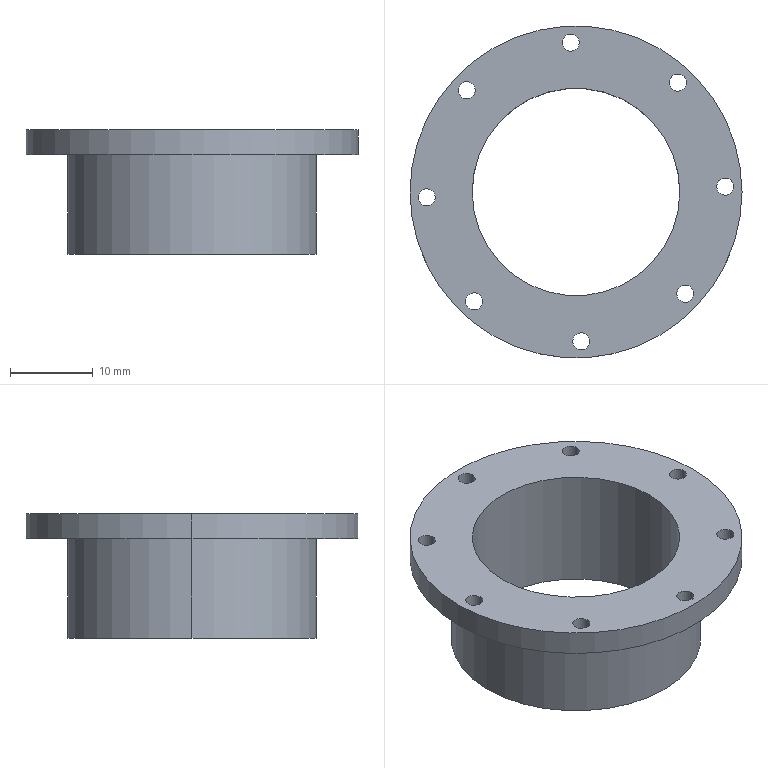Part | SolidWorks | features ICE 2, Cut 1, Extrusion 1 | 1 solid | 25 faces | box 40 x 40 x 15 mm | volume 4809 mm3 | cylinder 22 | plane 3 | commonest cylinder face diameters 2.06 x16 25 x2 30 x2 40 x2
STEP:
#1=CARTESIAN_POINT('',(16.959,0.6417,12.));
#2=VERTEX_POINT('',#1);
#3=CARTESIAN_POINT('',(19.019,0.6417,12.));
#4=VERTEX_POINT('',#3);
#5=CARTESIAN_POINT('',(17.989,0.6417,12.));
#6=DIRECTION('',(0.,0.,1.));
#7=DIRECTION('',(1.,0.,0.));
#8=AXIS2_PLACEMENT_3D('',#5,#6,#7);
#9=CIRCLE('',#8,1.03);
#10=EDGE_CURVE('',#2,#4,#9,.T.);
#11=ORIENTED_EDGE('',*,*,#10,.F.);
#12=CARTESIAN_POINT('',(16.959,0.6417,15.));
#13=VERTEX_POINT('',#12);
#14=CARTESIAN_POINT('',(16.959,0.6417,5.));
#15=DIRECTION('',(0.,0.,1.));
#16=VECTOR('',#15,1000.);
#17=LINE('',#14,#16);
#18=EDGE_CURVE('',#2,#13,#17,.T.);
#19=ORIENTED_EDGE('',*,*,#18,.T.);
#20=CARTESIAN_POINT('',(19.019,0.6417,15.));
#21=VERTEX_POINT('',#20);
#22=CARTESIAN_POINT('',(17.989,0.6417,15.));
#23=DIRECTION('',(0.,0.,1.));
#24=DIRECTION('',(1.,0.,0.));
#25=AXIS2_PLACEMENT_3D('',#22,#23,#24);
#26=CIRCLE('',#25,1.03);
#27=EDGE_CURVE('',#13,#21,#26,.T.);
#28=ORIENTED_EDGE('',*,*,#27,.T.);
#29=CARTESIAN_POINT('',(19.019,0.6417,5.));
#30=DIRECTION('',(0.,0.,1.));
#31=VECTOR('',#30,1000.);
#32=LINE('',#29,#31);
#33=EDGE_CURVE('',#4,#21,#32,.T.);
#34=ORIENTED_EDGE('',*,*,#33,.F.);
#35=EDGE_LOOP('',(#11,#19,#28,#34));
#36=FACE_OUTER_BOUND('',#35,.T.);
#37=CARTESIAN_POINT('',(17.989,0.6417,5.));
#38=DIRECTION('',(0.,0.,1.));
#39=DIRECTION('',(1.,0.,0.));
#40=AXIS2_PLACEMENT_3D('',#37,#38,#39);
#41=CYLINDRICAL_SURFACE('',#40,1.03);
#42=ADVANCED_FACE('',(#36),#41,.F.);
#43=CARTESIAN_POINT('',(12.144,-12.266,12.));
#44=VERTEX_POINT('',#43);
#45=CARTESIAN_POINT('',(14.204,-12.266,12.));
#46=VERTEX_POINT('',#45);
#47=CARTESIAN_POINT('',(13.174,-12.266,12.));
#48=DIRECTION('',(0.,0.,1.));
#49=DIRECTION('',(1.,0.,0.));
#50=AXIS2_PLACEMENT_3D('',#47,#48,#49);
#51=CIRCLE('',#50,1.03);
#52=EDGE_CURVE('',#44,#46,#51,.T.);
#53=ORIENTED_EDGE('',*,*,#52,.F.);
#54=CARTESIAN_POINT('',(12.144,-12.266,15.));
#55=VERTEX_POINT('',#54);
#56=CARTESIAN_POINT('',(12.144,-12.266,5.));
#57=DIRECTION('',(0.,0.,1.));
#58=VECTOR('',#57,1000.);
#59=LINE('',#56,#58);
#60=EDGE_CURVE('',#44,#55,#59,.T.);
#61=ORIENTED_EDGE('',*,*,#60,.T.);
#62=CARTESIAN_POINT('',(14.204,-12.266,15.));
#63=VERTEX_POINT('',#62);
#64=CARTESIAN_POINT('',(13.174,-12.266,15.));
#65=DIRECTION('',(0.,0.,1.));
#66=DIRECTION('',(1.,0.,0.));
#67=AXIS2_PLACEMENT_3D('',#64,#65,#66);
#68=CIRCLE('',#67,1.03);
#69=EDGE_CURVE('',#55,#63,#68,.T.);
#70=ORIENTED_EDGE('',*,*,#69,.T.);
#71=CARTESIAN_POINT('',(14.204,-12.266,5.));
#72=DIRECTION('',(0.,0.,1.));
#73=VECTOR('',#72,1000.);
#74=LINE('',#71,#73);
#75=EDGE_CURVE('',#46,#63,#74,.T.);
#76=ORIENTED_EDGE('',*,*,#75,.F.);
#77=EDGE_LOOP('',(#53,#61,#70,#76));
#78=FACE_OUTER_BOUND('',#77,.T.);
#79=CARTESIAN_POINT('',(13.174,-12.266,5.));
#80=DIRECTION('',(0.,0.,1.));
#81=DIRECTION('',(1.,0.,0.));
#82=AXIS2_PLACEMENT_3D('',#79,#80,#81);
#83=CYLINDRICAL_SURFACE('',#82,1.03);
#84=ADVANCED_FACE('',(#78),#83,.F.);
#85=CARTESIAN_POINT('',(-0.3883,-17.989,12.));
#86=VERTEX_POINT('',#85);
#87=CARTESIAN_POINT('',(1.672,-17.989,12.));
#88=VERTEX_POINT('',#87);
#89=CARTESIAN_POINT('',(0.6417,-17.989,12.));
#90=DIRECTION('',(0.,0.,1.));
#91=DIRECTION('',(1.,0.,0.));
#92=AXIS2_PLACEMENT_3D('',#89,#90,#91);
#93=CIRCLE('',#92,1.03);
#94=EDGE_CURVE('',#86,#88,#93,.T.);
#95=ORIENTED_EDGE('',*,*,#94,.F.);
#96=CARTESIAN_POINT('',(-0.3883,-17.989,15.));
#97=VERTEX_POINT('',#96);
#98=CARTESIAN_POINT('',(-0.3883,-17.989,5.));
#99=DIRECTION('',(0.,0.,1.));
#100=VECTOR('',#99,1000.);
#101=LINE('',#98,#100);
#102=EDGE_CURVE('',#86,#97,#101,.T.);
#103=ORIENTED_EDGE('',*,*,#102,.T.);
#104=CARTESIAN_POINT('',(1.672,-17.989,15.));
#105=VERTEX_POINT('',#104);
#106=CARTESIAN_POINT('',(0.6417,-17.989,15.));
#107=DIRECTION('',(0.,0.,1.));
#108=DIRECTION('',(1.,0.,0.));
#109=AXIS2_PLACEMENT_3D('',#106,#107,#108);
#110=CIRCLE('',#109,1.03);
#111=EDGE_CURVE('',#97,#105,#110,.T.);
#112=ORIENTED_EDGE('',*,*,#111,.T.);
#113=CARTESIAN_POINT('',(1.672,-17.989,5.));
#114=DIRECTION('',(0.,0.,1.));
#115=VECTOR('',#114,1000.);
#116=LINE('',#113,#115);
#117=EDGE_CURVE('',#88,#105,#116,.T.);
#118=ORIENTED_EDGE('',*,*,#117,.F.);
#119=EDGE_LOOP('',(#95,#103,#112,#118));
#120=FACE_OUTER_BOUND('',#119,.T.);
#121=CARTESIAN_POINT('',(0.6417,-17.989,5.));
#122=DIRECTION('',(0.,0.,1.));
#123=DIRECTION('',(1.,0.,0.));
#124=AXIS2_PLACEMENT_3D('',#121,#122,#123);
#125=CYLINDRICAL_SURFACE('',#124,1.03);
#126=ADVANCED_FACE('',(#120),#125,.F.);
#127=CARTESIAN_POINT('',(-13.296,-13.174,12.));
#128=VERTEX_POINT('',#127);
#129=CARTESIAN_POINT('',(-11.236,-13.174,12.));
#130=VERTEX_POINT('',#129);
#131=CARTESIAN_POINT('',(-12.266,-13.174,12.));
#132=DIRECTION('',(0.,0.,1.));
#133=DIRECTION('',(1.,0.,0.));
#134=AXIS2_PLACEMENT_3D('',#131,#132,#133);
#135=CIRCLE('',#134,1.03);
#136=EDGE_CURVE('',#128,#130,#135,.T.);
#137=ORIENTED_EDGE('',*,*,#136,.F.);
#138=CARTESIAN_POINT('',(-13.296,-13.174,15.));
#139=VERTEX_POINT('',#138);
#140=CARTESIAN_POINT('',(-13.296,-13.174,5.));
#141=DIRECTION('',(0.,0.,1.));
#142=VECTOR('',#141,1000.);
#143=LINE('',#140,#142);
#144=EDGE_CURVE('',#128,#139,#143,.T.);
#145=ORIENTED_EDGE('',*,*,#144,.T.);
#146=CARTESIAN_POINT('',(-11.236,-13.174,15.));
#147=VERTEX_POINT('',#146);
#148=CARTESIAN_POINT('',(-12.266,-13.174,15.));
#149=DIRECTION('',(0.,0.,1.));
#150=DIRECTION('',(1.,0.,0.));
#151=AXIS2_PLACEMENT_3D('',#148,#149,#150);
#152=CIRCLE('',#151,1.03);
#153=EDGE_CURVE('',#139,#147,#152,.T.);
#154=ORIENTED_EDGE('',*,*,#153,.T.);
#155=CARTESIAN_POINT('',(-11.236,-13.174,5.));
#156=DIRECTION('',(0.,0.,1.));
#157=VECTOR('',#156,1000.);
#158=LINE('',#155,#157);
#159=EDGE_CURVE('',#130,#147,#158,.T.);
#160=ORIENTED_EDGE('',*,*,#159,.F.);
#161=EDGE_LOOP('',(#137,#145,#154,#160));
#162=FACE_OUTER_BOUND('',#161,.T.);
#163=CARTESIAN_POINT('',(-12.266,-13.174,5.));
#164=DIRECTION('',(0.,0.,1.));
#165=DIRECTION('',(1.,0.,0.));
#166=AXIS2_PLACEMENT_3D('',#163,#164,#165);
#167=CYLINDRICAL_SURFACE('',#166,1.03);
#168=ADVANCED_FACE('',(#162),#167,.F.);
#169=CARTESIAN_POINT('',(-19.019,-0.6417,12.));
#170=VERTEX_POINT('',#169);
#171=CARTESIAN_POINT('',(-16.959,-0.6417,12.));
#172=VERTEX_POINT('',#171);
#173=CARTESIAN_POINT('',(-17.989,-0.6417,12.));
#174=DIRECTION('',(0.,0.,1.));
#175=DIRECTION('',(1.,0.,0.));
#176=AXIS2_PLACEMENT_3D('',#173,#174,#175);
#177=CIRCLE('',#176,1.03);
#178=EDGE_CURVE('',#170,#172,#177,.T.);
#179=ORIENTED_EDGE('',*,*,#178,.F.);
#180=CARTESIAN_POINT('',(-19.019,-0.6417,15.));
#181=VERTEX_POINT('',#180);
#182=CARTESIAN_POINT('',(-19.019,-0.6417,5.));
#183=DIRECTION('',(0.,0.,1.));
#184=VECTOR('',#183,1000.);
#185=LINE('',#182,#184);
#186=EDGE_CURVE('',#170,#181,#185,.T.);
#187=ORIENTED_EDGE('',*,*,#186,.T.);
#188=CARTESIAN_POINT('',(-16.959,-0.6417,15.));
#189=VERTEX_POINT('',#188);
#190=CARTESIAN_POINT('',(-17.989,-0.6417,15.));
#191=DIRECTION('',(0.,0.,1.));
#192=DIRECTION('',(1.,0.,0.));
#193=AXIS2_PLACEMENT_3D('',#190,#191,#192);
#194=CIRCLE('',#193,1.03);
#195=EDGE_CURVE('',#181,#189,#194,.T.);
#196=ORIENTED_EDGE('',*,*,#195,.T.);
#197=CARTESIAN_POINT('',(-16.959,-0.6417,5.));
#198=DIRECTION('',(0.,0.,1.));
#199=VECTOR('',#198,1000.);
#200=LINE('',#197,#199);
#201=EDGE_CURVE('',#172,#189,#200,.T.);
#202=ORIENTED_EDGE('',*,*,#201,.F.);
#203=EDGE_LOOP('',(#179,#187,#196,#202));
#204=FACE_OUTER_BOUND('',#203,.T.);
#205=CARTESIAN_POINT('',(-17.989,-0.6417,5.));
#206=DIRECTION('',(0.,0.,1.));
#207=DIRECTION('',(1.,0.,0.));
#208=AXIS2_PLACEMENT_3D('',#205,#206,#207);
#209=CYLINDRICAL_SURFACE('',#208,1.03);
#210=ADVANCED_FACE('',(#204),#209,.F.);
#211=CARTESIAN_POINT('',(-14.204,12.266,12.));
#212=VERTEX_POINT('',#211);
#213=CARTESIAN_POINT('',(-12.144,12.266,12.));
#214=VERTEX_POINT('',#213);
#215=CARTESIAN_POINT('',(-13.174,12.266,12.));
#216=DIRECTION('',(0.,0.,1.));
#217=DIRECTION('',(1.,0.,0.));
#218=AXIS2_PLACEMENT_3D('',#215,#216,#217);
#219=CIRCLE('',#218,1.03);
#220=EDGE_CURVE('',#212,#214,#219,.T.);
#221=ORIENTED_EDGE('',*,*,#220,.F.);
#222=CARTESIAN_POINT('',(-14.204,12.266,15.));
#223=VERTEX_POINT('',#222);
#224=CARTESIAN_POINT('',(-14.204,12.266,5.));
#225=DIRECTION('',(0.,0.,1.));
#226=VECTOR('',#225,1000.);
#227=LINE('',#224,#226);
#228=EDGE_CURVE('',#212,#223,#227,.T.);
#229=ORIENTED_EDGE('',*,*,#228,.T.);
#230=CARTESIAN_POINT('',(-12.144,12.266,15.));
#231=VERTEX_POINT('',#230);
#232=CARTESIAN_POINT('',(-13.174,12.266,15.));
#233=DIRECTION('',(0.,0.,1.));
#234=DIRECTION('',(1.,0.,0.));
#235=AXIS2_PLACEMENT_3D('',#232,#233,#234);
#236=CIRCLE('',#235,1.03);
#237=EDGE_CURVE('',#223,#231,#236,.T.);
#238=ORIENTED_EDGE('',*,*,#237,.T.);
#239=CARTESIAN_POINT('',(-12.144,12.266,5.));
#240=DIRECTION('',(0.,0.,1.));
#241=VECTOR('',#240,1000.);
#242=LINE('',#239,#241);
#243=EDGE_CURVE('',#214,#231,#242,.T.);
#244=ORIENTED_EDGE('',*,*,#243,.F.);
#245=EDGE_LOOP('',(#221,#229,#238,#244));
#246=FACE_OUTER_BOUND('',#245,.T.);
#247=CARTESIAN_POINT('',(-13.174,12.266,5.));
#248=DIRECTION('',(0.,0.,1.));
#249=DIRECTION('',(1.,0.,0.));
#250=AXIS2_PLACEMENT_3D('',#247,#248,#249);
#251=CYLINDRICAL_SURFACE('',#250,1.03);
#252=ADVANCED_FACE('',(#246),#251,.F.);
#253=CARTESIAN_POINT('',(-1.672,17.989,12.));
#254=VERTEX_POINT('',#253);
#255=CARTESIAN_POINT('',(0.3883,17.989,12.));
#256=VERTEX_POINT('',#255);
#257=CARTESIAN_POINT('',(-0.6417,17.989,12.));
#258=DIRECTION('',(0.,0.,1.));
#259=DIRECTION('',(1.,0.,0.));
#260=AXIS2_PLACEMENT_3D('',#257,#258,#259);
#261=CIRCLE('',#260,1.03);
#262=EDGE_CURVE('',#254,#256,#261,.T.);
#263=ORIENTED_EDGE('',*,*,#262,.F.);
#264=CARTESIAN_POINT('',(-1.672,17.989,15.));
#265=VERTEX_POINT('',#264);
#266=CARTESIAN_POINT('',(-1.672,17.989,5.));
#267=DIRECTION('',(0.,0.,1.));
#268=VECTOR('',#267,1000.);
#269=LINE('',#266,#268);
#270=EDGE_CURVE('',#254,#265,#269,.T.);
#271=ORIENTED_EDGE('',*,*,#270,.T.);
#272=CARTESIAN_POINT('',(0.3883,17.989,15.));
#273=VERTEX_POINT('',#272);
#274=CARTESIAN_POINT('',(-0.6417,17.989,15.));
#275=DIRECTION('',(0.,0.,1.));
#276=DIRECTION('',(1.,0.,0.));
#277=AXIS2_PLACEMENT_3D('',#274,#275,#276);
#278=CIRCLE('',#277,1.03);
#279=EDGE_CURVE('',#265,#273,#278,.T.);
#280=ORIENTED_EDGE('',*,*,#279,.T.);
#281=CARTESIAN_POINT('',(0.3883,17.989,5.));
#282=DIRECTION('',(0.,0.,1.));
#283=VECTOR('',#282,1000.);
#284=LINE('',#281,#283);
#285=EDGE_CURVE('',#256,#273,#284,.T.);
#286=ORIENTED_EDGE('',*,*,#285,.F.);
#287=EDGE_LOOP('',(#263,#271,#280,#286));
#288=FACE_OUTER_BOUND('',#287,.T.);
#289=CARTESIAN_POINT('',(-0.6417,17.989,5.));
#290=DIRECTION('',(0.,0.,1.));
#291=DIRECTION('',(1.,0.,0.));
#292=AXIS2_PLACEMENT_3D('',#289,#290,#291);
#293=CYLINDRICAL_SURFACE('',#292,1.03);
#294=ADVANCED_FACE('',(#288),#293,.F.);
#295=CARTESIAN_POINT('',(11.236,13.174,12.));
#296=VERTEX_POINT('',#295);
#297=CARTESIAN_POINT('',(13.296,13.174,12.));
#298=VERTEX_POINT('',#297);
#299=CARTESIAN_POINT('',(12.266,13.174,12.));
#300=DIRECTION('',(0.,0.,1.));
#301=DIRECTION('',(1.,0.,0.));
#302=AXIS2_PLACEMENT_3D('',#299,#300,#301);
#303=CIRCLE('',#302,1.03);
#304=EDGE_CURVE('',#296,#298,#303,.T.);
#305=ORIENTED_EDGE('',*,*,#304,.F.);
#306=CARTESIAN_POINT('',(11.236,13.174,15.));
#307=VERTEX_POINT('',#306);
#308=CARTESIAN_POINT('',(11.236,13.174,5.));
#309=DIRECTION('',(0.,0.,1.));
#310=VECTOR('',#309,1000.);
#311=LINE('',#308,#310);
#312=EDGE_CURVE('',#296,#307,#311,.T.);
#313=ORIENTED_EDGE('',*,*,#312,.T.);
#314=CARTESIAN_POINT('',(13.296,13.174,15.));
#315=VERTEX_POINT('',#314);
#316=CARTESIAN_POINT('',(12.266,13.174,15.));
#317=DIRECTION('',(0.,0.,1.));
#318=DIRECTION('',(1.,0.,0.));
#319=AXIS2_PLACEMENT_3D('',#316,#317,#318);
#320=CIRCLE('',#319,1.03);
#321=EDGE_CURVE('',#307,#315,#320,.T.);
#322=ORIENTED_EDGE('',*,*,#321,.T.);
#323=CARTESIAN_POINT('',(13.296,13.174,5.));
#324=DIRECTION('',(0.,0.,1.));
#325=VECTOR('',#324,1000.);
#326=LINE('',#323,#325);
#327=EDGE_CURVE('',#298,#315,#326,.T.);
#328=ORIENTED_EDGE('',*,*,#327,.F.);
#329=EDGE_LOOP('',(#305,#313,#322,#328));
#330=FACE_OUTER_BOUND('',#329,.T.);
#331=CARTESIAN_POINT('',(12.266,13.174,5.));
#332=DIRECTION('',(0.,0.,1.));
#333=DIRECTION('',(1.,0.,0.));
#334=AXIS2_PLACEMENT_3D('',#331,#332,#333);
#335=CYLINDRICAL_SURFACE('',#334,1.03);
#336=ADVANCED_FACE('',(#330),#335,.F.);
#337=CARTESIAN_POINT('',(20.,0.,15.));
#338=VERTEX_POINT('',#337);
#339=CARTESIAN_POINT('',(-20.,0.,15.));
#340=VERTEX_POINT('',#339);
#341=CARTESIAN_POINT('',(0.,0.,15.));
#342=DIRECTION('',(0.,0.,1.));
#343=DIRECTION('',(1.,0.,0.));
#344=AXIS2_PLACEMENT_3D('',#341,#342,#343);
#345=CIRCLE('',#344,20.);
#346=EDGE_CURVE('',#338,#340,#345,.T.);
#347=ORIENTED_EDGE('',*,*,#346,.F.);
#348=CARTESIAN_POINT('',(20.,0.,12.));
#349=VERTEX_POINT('',#348);
#350=CARTESIAN_POINT('',(20.,0.,71.569));
#351=DIRECTION('',(0.,0.,-1.));
#352=VECTOR('',#351,1000.);
#353=LINE('',#350,#352);
#354=EDGE_CURVE('',#338,#349,#353,.T.);
#355=ORIENTED_EDGE('',*,*,#354,.T.);
#356=CARTESIAN_POINT('',(-20.,0.,12.));
#357=VERTEX_POINT('',#356);
#358=CARTESIAN_POINT('',(0.,0.,12.));
#359=DIRECTION('',(0.,0.,1.));
#360=DIRECTION('',(1.,0.,0.));
#361=AXIS2_PLACEMENT_3D('',#358,#359,#360);
#362=CIRCLE('',#361,20.);
#363=EDGE_CURVE('',#349,#357,#362,.T.);
#364=ORIENTED_EDGE('',*,*,#363,.T.);
#365=CARTESIAN_POINT('',(-20.,0.,71.569));
#366=DIRECTION('',(0.,0.,-1.));
#367=VECTOR('',#366,1000.);
#368=LINE('',#365,#367);
#369=EDGE_CURVE('',#340,#357,#368,.T.);
#370=ORIENTED_EDGE('',*,*,#369,.F.);
#371=EDGE_LOOP('',(#347,#355,#364,#370));
#372=FACE_OUTER_BOUND('',#371,.T.);
#373=CARTESIAN_POINT('',(0.,0.,71.569));
#374=DIRECTION('',(0.,0.,-1.));
#375=DIRECTION('',(-1.,0.,0.));
#376=AXIS2_PLACEMENT_3D('',#373,#374,#375);
#377=CYLINDRICAL_SURFACE('',#376,20.);
#378=ADVANCED_FACE('',(#372),#377,.T.);
#379=CARTESIAN_POINT('',(-12.5,0.,15.));
#380=VERTEX_POINT('',#379);
#381=CARTESIAN_POINT('',(12.5,0.,15.));
#382=VERTEX_POINT('',#381);
#383=CARTESIAN_POINT('',(0.,0.,15.));
#384=DIRECTION('',(0.,0.,1.));
#385=DIRECTION('',(1.,0.,0.));
#386=AXIS2_PLACEMENT_3D('',#383,#384,#385);
#387=CIRCLE('',#386,12.5);
#388=EDGE_CURVE('',#380,#382,#387,.T.);
#389=ORIENTED_EDGE('',*,*,#388,.T.);
#390=CARTESIAN_POINT('',(12.5,0.,0.));
#391=VERTEX_POINT('',#390);
#392=CARTESIAN_POINT('',(12.5,0.,5.));
#393=DIRECTION('',(0.,0.,-1.));
#394=VECTOR('',#393,1000.);
#395=LINE('',#392,#394);
#396=EDGE_CURVE('',#382,#391,#395,.T.);
#397=ORIENTED_EDGE('',*,*,#396,.T.);
#398=CARTESIAN_POINT('',(-12.5,0.,0.));
#399=VERTEX_POINT('',#398);
#400=CARTESIAN_POINT('',(0.,0.,0.));
#401=DIRECTION('',(0.,0.,1.));
#402=DIRECTION('',(1.,0.,0.));
#403=AXIS2_PLACEMENT_3D('',#400,#401,#402);
#404=CIRCLE('',#403,12.5);
#405=EDGE_CURVE('',#399,#391,#404,.T.);
#406=ORIENTED_EDGE('',*,*,#405,.F.);
#407=CARTESIAN_POINT('',(-12.5,0.,5.));
#408=DIRECTION('',(0.,0.,-1.));
#409=VECTOR('',#408,1000.);
#410=LINE('',#407,#409);
#411=EDGE_CURVE('',#380,#399,#410,.T.);
#412=ORIENTED_EDGE('',*,*,#411,.F.);
#413=EDGE_LOOP('',(#389,#397,#406,#412));
#414=FACE_OUTER_BOUND('',#413,.T.);
#415=CARTESIAN_POINT('',(0.,0.,5.));
#416=DIRECTION('',(0.,0.,-1.));
#417=DIRECTION('',(-1.,0.,0.));
#418=AXIS2_PLACEMENT_3D('',#415,#416,#417);
#419=CYLINDRICAL_SURFACE('',#418,12.5);
#420=ADVANCED_FACE('',(#414),#419,.F.);
#421=CARTESIAN_POINT('',(15.,0.,12.));
#422=VERTEX_POINT('',#421);
#423=CARTESIAN_POINT('',(-15.,0.,12.));
#424=VERTEX_POINT('',#423);
#425=CARTESIAN_POINT('',(0.,0.,12.));
#426=DIRECTION('',(0.,0.,1.));
#427=DIRECTION('',(1.,0.,0.));
#428=AXIS2_PLACEMENT_3D('',#425,#426,#427);
#429=CIRCLE('',#428,15.);
#430=EDGE_CURVE('',#422,#424,#429,.T.);
#431=ORIENTED_EDGE('',*,*,#430,.F.);
#432=CARTESIAN_POINT('',(15.,0.,0.));
#433=VERTEX_POINT('',#432);
#434=CARTESIAN_POINT('',(15.,0.,5.));
#435=DIRECTION('',(0.,0.,-1.));
#436=VECTOR('',#435,1000.);
#437=LINE('',#434,#436);
#438=EDGE_CURVE('',#422,#433,#437,.T.);
#439=ORIENTED_EDGE('',*,*,#438,.T.);
#440=CARTESIAN_POINT('',(-15.,0.,0.));
#441=VERTEX_POINT('',#440);
#442=CARTESIAN_POINT('',(0.,0.,0.));
#443=DIRECTION('',(0.,0.,1.));
#444=DIRECTION('',(1.,0.,0.));
#445=AXIS2_PLACEMENT_3D('',#442,#443,#444);
#446=CIRCLE('',#445,15.);
#447=EDGE_CURVE('',#433,#441,#446,.T.);
#448=ORIENTED_EDGE('',*,*,#447,.T.);
#449=CARTESIAN_POINT('',(-15.,0.,5.));
#450=DIRECTION('',(0.,0.,-1.));
#451=VECTOR('',#450,1000.);
#452=LINE('',#449,#451);
#453=EDGE_CURVE('',#424,#441,#452,.T.);
#454=ORIENTED_EDGE('',*,*,#453,.F.);
#455=EDGE_LOOP('',(#431,#439,#448,#454));
#456=FACE_OUTER_BOUND('',#455,.T.);
#457=CARTESIAN_POINT('',(0.,0.,5.));
#458=DIRECTION('',(0.,0.,-1.));
#459=DIRECTION('',(-1.,0.,0.));
#460=AXIS2_PLACEMENT_3D('',#457,#458,#459);
#461=CYLINDRICAL_SURFACE('',#460,15.);
#462=ADVANCED_FACE('',(#456),#461,.T.);
#463=ORIENTED_EDGE('',*,*,#438,.F.);
#464=CARTESIAN_POINT('',(0.,0.,12.));
#465=DIRECTION('',(0.,0.,1.));
#466=DIRECTION('',(1.,0.,0.));
#467=AXIS2_PLACEMENT_3D('',#464,#465,#466);
#468=CIRCLE('',#467,15.);
#469=EDGE_CURVE('',#424,#422,#468,.T.);
#470=ORIENTED_EDGE('',*,*,#469,.F.);
#471=ORIENTED_EDGE('',*,*,#453,.T.);
#472=CARTESIAN_POINT('',(0.,0.,0.));
#473=DIRECTION('',(0.,0.,1.));
#474=DIRECTION('',(1.,0.,0.));
#475=AXIS2_PLACEMENT_3D('',#472,#473,#474);
#476=CIRCLE('',#475,15.);
#477=EDGE_CURVE('',#441,#433,#476,.T.);
#478=ORIENTED_EDGE('',*,*,#477,.T.);
#479=EDGE_LOOP('',(#463,#470,#471,#478));
#480=FACE_OUTER_BOUND('',#479,.T.);
#481=CARTESIAN_POINT('',(0.,0.,5.));
#482=DIRECTION('',(0.,0.,-1.));
#483=DIRECTION('',(-1.,0.,0.));
#484=AXIS2_PLACEMENT_3D('',#481,#482,#483);
#485=CYLINDRICAL_SURFACE('',#484,15.);
#486=ADVANCED_FACE('',(#480),#485,.T.);
#487=ORIENTED_EDGE('',*,*,#477,.F.);
#488=ORIENTED_EDGE('',*,*,#447,.F.);
#489=EDGE_LOOP('',(#487,#488));
#490=FACE_OUTER_BOUND('',#489,.T.);
#491=ORIENTED_EDGE('',*,*,#405,.T.);
#492=CARTESIAN_POINT('',(0.,0.,0.));
#493=DIRECTION('',(0.,0.,1.));
#494=DIRECTION('',(1.,0.,0.));
#495=AXIS2_PLACEMENT_3D('',#492,#493,#494);
#496=CIRCLE('',#495,12.5);
#497=EDGE_CURVE('',#391,#399,#496,.T.);
#498=ORIENTED_EDGE('',*,*,#497,.T.);
#499=EDGE_LOOP('',(#491,#498));
#500=FACE_BOUND('',#499,.T.);
#501=CARTESIAN_POINT('',(0.,0.,0.));
#502=DIRECTION('',(0.,0.,1.));
#503=DIRECTION('',(1.,0.,0.));
#504=AXIS2_PLACEMENT_3D('',#501,#502,#503);
#505=PLANE('',#504);
#506=ADVANCED_FACE('',(#490,#500),#505,.F.);
#507=ORIENTED_EDGE('',*,*,#396,.F.);
#508=CARTESIAN_POINT('',(0.,0.,15.));
#509=DIRECTION('',(0.,0.,1.));
#510=DIRECTION('',(1.,0.,0.));
#511=AXIS2_PLACEMENT_3D('',#508,#509,#510);
#512=CIRCLE('',#511,12.5);
#513=EDGE_CURVE('',#382,#380,#512,.T.);
#514=ORIENTED_EDGE('',*,*,#513,.T.);
#515=ORIENTED_EDGE('',*,*,#411,.T.);
#516=ORIENTED_EDGE('',*,*,#497,.F.);
#517=EDGE_LOOP('',(#507,#514,#515,#516));
#518=FACE_OUTER_BOUND('',#517,.T.);
#519=CARTESIAN_POINT('',(0.,0.,5.));
#520=DIRECTION('',(0.,0.,-1.));
#521=DIRECTION('',(-1.,0.,0.));
#522=AXIS2_PLACEMENT_3D('',#519,#520,#521);
#523=CYLINDRICAL_SURFACE('',#522,12.5);
#524=ADVANCED_FACE('',(#518),#523,.F.);
#525=CARTESIAN_POINT('',(17.989,0.6417,15.));
#526=DIRECTION('',(0.,0.,1.));
#527=DIRECTION('',(1.,0.,0.));
#528=AXIS2_PLACEMENT_3D('',#525,#526,#527);
#529=CIRCLE('',#528,1.03);
#530=EDGE_CURVE('',#21,#13,#529,.T.);
#531=ORIENTED_EDGE('',*,*,#530,.F.);
#532=ORIENTED_EDGE('',*,*,#27,.F.);
#533=EDGE_LOOP('',(#531,#532));
#534=FACE_BOUND('',#533,.T.);
#535=CARTESIAN_POINT('',(13.174,-12.266,15.));
#536=DIRECTION('',(0.,0.,1.));
#537=DIRECTION('',(1.,0.,0.));
#538=AXIS2_PLACEMENT_3D('',#535,#536,#537);
#539=CIRCLE('',#538,1.03);
#540=EDGE_CURVE('',#63,#55,#539,.T.);
#541=ORIENTED_EDGE('',*,*,#540,.F.);
#542=ORIENTED_EDGE('',*,*,#69,.F.);
#543=EDGE_LOOP('',(#541,#542));
#544=FACE_BOUND('',#543,.T.);
#545=CARTESIAN_POINT('',(0.6417,-17.989,15.));
#546=DIRECTION('',(0.,0.,1.));
#547=DIRECTION('',(1.,0.,0.));
#548=AXIS2_PLACEMENT_3D('',#545,#546,#547);
#549=CIRCLE('',#548,1.03);
#550=EDGE_CURVE('',#105,#97,#549,.T.);
#551=ORIENTED_EDGE('',*,*,#550,.F.);
#552=ORIENTED_EDGE('',*,*,#111,.F.);
#553=EDGE_LOOP('',(#551,#552));
#554=FACE_BOUND('',#553,.T.);
#555=CARTESIAN_POINT('',(-12.266,-13.174,15.));
#556=DIRECTION('',(0.,0.,1.));
#557=DIRECTION('',(1.,0.,0.));
#558=AXIS2_PLACEMENT_3D('',#555,#556,#557);
#559=CIRCLE('',#558,1.03);
#560=EDGE_CURVE('',#147,#139,#559,.T.);
#561=ORIENTED_EDGE('',*,*,#560,.F.);
#562=ORIENTED_EDGE('',*,*,#153,.F.);
#563=EDGE_LOOP('',(#561,#562));
#564=FACE_BOUND('',#563,.T.);
#565=CARTESIAN_POINT('',(-17.989,-0.6417,15.));
#566=DIRECTION('',(0.,0.,1.));
#567=DIRECTION('',(1.,0.,0.));
#568=AXIS2_PLACEMENT_3D('',#565,#566,#567);
#569=CIRCLE('',#568,1.03);
#570=EDGE_CURVE('',#189,#181,#569,.T.);
#571=ORIENTED_EDGE('',*,*,#570,.F.);
#572=ORIENTED_EDGE('',*,*,#195,.F.);
#573=EDGE_LOOP('',(#571,#572));
#574=FACE_BOUND('',#573,.T.);
#575=CARTESIAN_POINT('',(-13.174,12.266,15.));
#576=DIRECTION('',(0.,0.,1.));
#577=DIRECTION('',(1.,0.,0.));
#578=AXIS2_PLACEMENT_3D('',#575,#576,#577);
#579=CIRCLE('',#578,1.03);
#580=EDGE_CURVE('',#231,#223,#579,.T.);
#581=ORIENTED_EDGE('',*,*,#580,.F.);
#582=ORIENTED_EDGE('',*,*,#237,.F.);
#583=EDGE_LOOP('',(#581,#582));
#584=FACE_BOUND('',#583,.T.);
#585=CARTESIAN_POINT('',(-0.6417,17.989,15.));
#586=DIRECTION('',(0.,0.,1.));
#587=DIRECTION('',(1.,0.,0.));
#588=AXIS2_PLACEMENT_3D('',#585,#586,#587);
#589=CIRCLE('',#588,1.03);
#590=EDGE_CURVE('',#273,#265,#589,.T.);
#591=ORIENTED_EDGE('',*,*,#590,.F.);
#592=ORIENTED_EDGE('',*,*,#279,.F.);
#593=EDGE_LOOP('',(#591,#592));
#594=FACE_BOUND('',#593,.T.);
#595=CARTESIAN_POINT('',(12.266,13.174,15.));
#596=DIRECTION('',(0.,0.,1.));
#597=DIRECTION('',(1.,0.,0.));
#598=AXIS2_PLACEMENT_3D('',#595,#596,#597);
#599=CIRCLE('',#598,1.03);
#600=EDGE_CURVE('',#315,#307,#599,.T.);
#601=ORIENTED_EDGE('',*,*,#600,.F.);
#602=ORIENTED_EDGE('',*,*,#321,.F.);
#603=EDGE_LOOP('',(#601,#602));
#604=FACE_BOUND('',#603,.T.);
#605=ORIENTED_EDGE('',*,*,#388,.F.);
#606=ORIENTED_EDGE('',*,*,#513,.F.);
#607=EDGE_LOOP('',(#605,#606));
#608=FACE_BOUND('',#607,.T.);
#609=CARTESIAN_POINT('',(0.,0.,15.));
#610=DIRECTION('',(0.,0.,1.));
#611=DIRECTION('',(1.,0.,0.));
#612=AXIS2_PLACEMENT_3D('',#609,#610,#611);
#613=CIRCLE('',#612,20.);
#614=EDGE_CURVE('',#340,#338,#613,.T.);
#615=ORIENTED_EDGE('',*,*,#614,.T.);
#616=ORIENTED_EDGE('',*,*,#346,.T.);
#617=EDGE_LOOP('',(#615,#616));
#618=FACE_OUTER_BOUND('',#617,.T.);
#619=CARTESIAN_POINT('',(0.,0.,15.));
#620=DIRECTION('',(0.,0.,1.));
#621=DIRECTION('',(1.,0.,0.));
#622=AXIS2_PLACEMENT_3D('',#619,#620,#621);
#623=PLANE('',#622);
#624=ADVANCED_FACE('',(#534,#544,#554,#564,#574,#584,#594,#604,#608,#618),#623,.T.);
#625=ORIENTED_EDGE('',*,*,#354,.F.);
#626=ORIENTED_EDGE('',*,*,#614,.F.);
#627=ORIENTED_EDGE('',*,*,#369,.T.);
#628=CARTESIAN_POINT('',(0.,0.,12.));
#629=DIRECTION('',(0.,0.,1.));
#630=DIRECTION('',(1.,0.,0.));
#631=AXIS2_PLACEMENT_3D('',#628,#629,#630);
#632=CIRCLE('',#631,20.);
#633=EDGE_CURVE('',#357,#349,#632,.T.);
#634=ORIENTED_EDGE('',*,*,#633,.T.);
#635=EDGE_LOOP('',(#625,#626,#627,#634));
#636=FACE_OUTER_BOUND('',#635,.T.);
#637=CARTESIAN_POINT('',(0.,0.,71.569));
#638=DIRECTION('',(0.,0.,-1.));
#639=DIRECTION('',(-1.,0.,0.));
#640=AXIS2_PLACEMENT_3D('',#637,#638,#639);
#641=CYLINDRICAL_SURFACE('',#640,20.);
#642=ADVANCED_FACE('',(#636),#641,.T.);
#643=CARTESIAN_POINT('',(17.989,0.6417,12.));
#644=DIRECTION('',(0.,0.,1.));
#645=DIRECTION('',(1.,0.,0.));
#646=AXIS2_PLACEMENT_3D('',#643,#644,#645);
#647=CIRCLE('',#646,1.03);
#648=EDGE_CURVE('',#4,#2,#647,.T.);
#649=ORIENTED_EDGE('',*,*,#648,.T.);
#650=ORIENTED_EDGE('',*,*,#10,.T.);
#651=EDGE_LOOP('',(#649,#650));
#652=FACE_BOUND('',#651,.T.);
#653=CARTESIAN_POINT('',(13.174,-12.266,12.));
#654=DIRECTION('',(0.,0.,1.));
#655=DIRECTION('',(1.,0.,0.));
#656=AXIS2_PLACEMENT_3D('',#653,#654,#655);
#657=CIRCLE('',#656,1.03);
#658=EDGE_CURVE('',#46,#44,#657,.T.);
#659=ORIENTED_EDGE('',*,*,#658,.T.);
#660=ORIENTED_EDGE('',*,*,#52,.T.);
#661=EDGE_LOOP('',(#659,#660));
#662=FACE_BOUND('',#661,.T.);
#663=CARTESIAN_POINT('',(0.6417,-17.989,12.));
#664=DIRECTION('',(0.,0.,1.));
#665=DIRECTION('',(1.,0.,0.));
#666=AXIS2_PLACEMENT_3D('',#663,#664,#665);
#667=CIRCLE('',#666,1.03);
#668=EDGE_CURVE('',#88,#86,#667,.T.);
#669=ORIENTED_EDGE('',*,*,#668,.T.);
#670=ORIENTED_EDGE('',*,*,#94,.T.);
#671=EDGE_LOOP('',(#669,#670));
#672=FACE_BOUND('',#671,.T.);
#673=CARTESIAN_POINT('',(-12.266,-13.174,12.));
#674=DIRECTION('',(0.,0.,1.));
#675=DIRECTION('',(1.,0.,0.));
#676=AXIS2_PLACEMENT_3D('',#673,#674,#675);
#677=CIRCLE('',#676,1.03);
#678=EDGE_CURVE('',#130,#128,#677,.T.);
#679=ORIENTED_EDGE('',*,*,#678,.T.);
#680=ORIENTED_EDGE('',*,*,#136,.T.);
#681=EDGE_LOOP('',(#679,#680));
#682=FACE_BOUND('',#681,.T.);
#683=CARTESIAN_POINT('',(-17.989,-0.6417,12.));
#684=DIRECTION('',(0.,0.,1.));
#685=DIRECTION('',(1.,0.,0.));
#686=AXIS2_PLACEMENT_3D('',#683,#684,#685);
#687=CIRCLE('',#686,1.03);
#688=EDGE_CURVE('',#172,#170,#687,.T.);
#689=ORIENTED_EDGE('',*,*,#688,.T.);
#690=ORIENTED_EDGE('',*,*,#178,.T.);
#691=EDGE_LOOP('',(#689,#690));
#692=FACE_BOUND('',#691,.T.);
#693=CARTESIAN_POINT('',(-13.174,12.266,12.));
#694=DIRECTION('',(0.,0.,1.));
#695=DIRECTION('',(1.,0.,0.));
#696=AXIS2_PLACEMENT_3D('',#693,#694,#695);
#697=CIRCLE('',#696,1.03);
#698=EDGE_CURVE('',#214,#212,#697,.T.);
#699=ORIENTED_EDGE('',*,*,#698,.T.);
#700=ORIENTED_EDGE('',*,*,#220,.T.);
#701=EDGE_LOOP('',(#699,#700));
#702=FACE_BOUND('',#701,.T.);
#703=CARTESIAN_POINT('',(-0.6417,17.989,12.));
#704=DIRECTION('',(0.,0.,1.));
#705=DIRECTION('',(1.,0.,0.));
#706=AXIS2_PLACEMENT_3D('',#703,#704,#705);
#707=CIRCLE('',#706,1.03);
#708=EDGE_CURVE('',#256,#254,#707,.T.);
#709=ORIENTED_EDGE('',*,*,#708,.T.);
#710=ORIENTED_EDGE('',*,*,#262,.T.);
#711=EDGE_LOOP('',(#709,#710));
#712=FACE_BOUND('',#711,.T.);
#713=CARTESIAN_POINT('',(12.266,13.174,12.));
#714=DIRECTION('',(0.,0.,1.));
#715=DIRECTION('',(1.,0.,0.));
#716=AXIS2_PLACEMENT_3D('',#713,#714,#715);
#717=CIRCLE('',#716,1.03);
#718=EDGE_CURVE('',#298,#296,#717,.T.);
#719=ORIENTED_EDGE('',*,*,#718,.T.);
#720=ORIENTED_EDGE('',*,*,#304,.T.);
#721=EDGE_LOOP('',(#719,#720));
#722=FACE_BOUND('',#721,.T.);
#723=ORIENTED_EDGE('',*,*,#469,.T.);
#724=ORIENTED_EDGE('',*,*,#430,.T.);
#725=EDGE_LOOP('',(#723,#724));
#726=FACE_BOUND('',#725,.T.);
#727=ORIENTED_EDGE('',*,*,#633,.F.);
#728=ORIENTED_EDGE('',*,*,#363,.F.);
#729=EDGE_LOOP('',(#727,#728));
#730=FACE_OUTER_BOUND('',#729,.T.);
#731=CARTESIAN_POINT('',(0.,0.,12.));
#732=DIRECTION('',(0.,0.,1.));
#733=DIRECTION('',(1.,0.,0.));
#734=AXIS2_PLACEMENT_3D('',#731,#732,#733);
#735=PLANE('',#734);
#736=ADVANCED_FACE('',(#652,#662,#672,#682,#692,#702,#712,#722,#726,#730),#735,.F.);
#737=ORIENTED_EDGE('',*,*,#312,.F.);
#738=ORIENTED_EDGE('',*,*,#718,.F.);
#739=ORIENTED_EDGE('',*,*,#327,.T.);
#740=ORIENTED_EDGE('',*,*,#600,.T.);
#741=EDGE_LOOP('',(#737,#738,#739,#740));
#742=FACE_OUTER_BOUND('',#741,.T.);
#743=CARTESIAN_POINT('',(12.266,13.174,5.));
#744=DIRECTION('',(0.,0.,1.));
#745=DIRECTION('',(1.,0.,0.));
#746=AXIS2_PLACEMENT_3D('',#743,#744,#745);
#747=CYLINDRICAL_SURFACE('',#746,1.03);
#748=ADVANCED_FACE('',(#742),#747,.F.);
#749=ORIENTED_EDGE('',*,*,#270,.F.);
#750=ORIENTED_EDGE('',*,*,#708,.F.);
#751=ORIENTED_EDGE('',*,*,#285,.T.);
#752=ORIENTED_EDGE('',*,*,#590,.T.);
#753=EDGE_LOOP('',(#749,#750,#751,#752));
#754=FACE_OUTER_BOUND('',#753,.T.);
#755=CARTESIAN_POINT('',(-0.6417,17.989,5.));
#756=DIRECTION('',(0.,0.,1.));
#757=DIRECTION('',(1.,0.,0.));
#758=AXIS2_PLACEMENT_3D('',#755,#756,#757);
#759=CYLINDRICAL_SURFACE('',#758,1.03);
#760=ADVANCED_FACE('',(#754),#759,.F.);
#761=ORIENTED_EDGE('',*,*,#228,.F.);
#762=ORIENTED_EDGE('',*,*,#698,.F.);
#763=ORIENTED_EDGE('',*,*,#243,.T.);
#764=ORIENTED_EDGE('',*,*,#580,.T.);
#765=EDGE_LOOP('',(#761,#762,#763,#764));
#766=FACE_OUTER_BOUND('',#765,.T.);
#767=CARTESIAN_POINT('',(-13.174,12.266,5.));
#768=DIRECTION('',(0.,0.,1.));
#769=DIRECTION('',(1.,0.,0.));
#770=AXIS2_PLACEMENT_3D('',#767,#768,#769);
#771=CYLINDRICAL_SURFACE('',#770,1.03);
#772=ADVANCED_FACE('',(#766),#771,.F.);
#773=ORIENTED_EDGE('',*,*,#186,.F.);
#774=ORIENTED_EDGE('',*,*,#688,.F.);
#775=ORIENTED_EDGE('',*,*,#201,.T.);
#776=ORIENTED_EDGE('',*,*,#570,.T.);
#777=EDGE_LOOP('',(#773,#774,#775,#776));
#778=FACE_OUTER_BOUND('',#777,.T.);
#779=CARTESIAN_POINT('',(-17.989,-0.6417,5.));
#780=DIRECTION('',(0.,0.,1.));
#781=DIRECTION('',(1.,0.,0.));
#782=AXIS2_PLACEMENT_3D('',#779,#780,#781);
#783=CYLINDRICAL_SURFACE('',#782,1.03);
#784=ADVANCED_FACE('',(#778),#783,.F.);
#785=ORIENTED_EDGE('',*,*,#144,.F.);
#786=ORIENTED_EDGE('',*,*,#678,.F.);
#787=ORIENTED_EDGE('',*,*,#159,.T.);
#788=ORIENTED_EDGE('',*,*,#560,.T.);
#789=EDGE_LOOP('',(#785,#786,#787,#788));
#790=FACE_OUTER_BOUND('',#789,.T.);
#791=CARTESIAN_POINT('',(-12.266,-13.174,5.));
#792=DIRECTION('',(0.,0.,1.));
#793=DIRECTION('',(1.,0.,0.));
#794=AXIS2_PLACEMENT_3D('',#791,#792,#793);
#795=CYLINDRICAL_SURFACE('',#794,1.03);
#796=ADVANCED_FACE('',(#790),#795,.F.);
#797=ORIENTED_EDGE('',*,*,#102,.F.);
#798=ORIENTED_EDGE('',*,*,#668,.F.);
#799=ORIENTED_EDGE('',*,*,#117,.T.);
#800=ORIENTED_EDGE('',*,*,#550,.T.);
#801=EDGE_LOOP('',(#797,#798,#799,#800));
#802=FACE_OUTER_BOUND('',#801,.T.);
#803=CARTESIAN_POINT('',(0.6417,-17.989,5.));
#804=DIRECTION('',(0.,0.,1.));
#805=DIRECTION('',(1.,0.,0.));
#806=AXIS2_PLACEMENT_3D('',#803,#804,#805);
#807=CYLINDRICAL_SURFACE('',#806,1.03);
#808=ADVANCED_FACE('',(#802),#807,.F.);
#809=ORIENTED_EDGE('',*,*,#60,.F.);
#810=ORIENTED_EDGE('',*,*,#658,.F.);
#811=ORIENTED_EDGE('',*,*,#75,.T.);
#812=ORIENTED_EDGE('',*,*,#540,.T.);
#813=EDGE_LOOP('',(#809,#810,#811,#812));
#814=FACE_OUTER_BOUND('',#813,.T.);
#815=CARTESIAN_POINT('',(13.174,-12.266,5.));
#816=DIRECTION('',(0.,0.,1.));
#817=DIRECTION('',(1.,0.,0.));
#818=AXIS2_PLACEMENT_3D('',#815,#816,#817);
#819=CYLINDRICAL_SURFACE('',#818,1.03);
#820=ADVANCED_FACE('',(#814),#819,.F.);
#821=ORIENTED_EDGE('',*,*,#18,.F.);
#822=ORIENTED_EDGE('',*,*,#648,.F.);
#823=ORIENTED_EDGE('',*,*,#33,.T.);
#824=ORIENTED_EDGE('',*,*,#530,.T.);
#825=EDGE_LOOP('',(#821,#822,#823,#824));
#826=FACE_OUTER_BOUND('',#825,.T.);
#827=CARTESIAN_POINT('',(17.989,0.6417,5.));
#828=DIRECTION('',(0.,0.,1.));
#829=DIRECTION('',(1.,0.,0.));
#830=AXIS2_PLACEMENT_3D('',#827,#828,#829);
#831=CYLINDRICAL_SURFACE('',#830,1.03);
#832=ADVANCED_FACE('',(#826),#831,.F.);
#833=CLOSED_SHELL('',(#42,#84,#126,#168,#210,#252,#294,#336,#378,#420,#462,#486,#506,#524,#624,#642,#736,#748,#760,#772,#784,#796,#808,#820,#832));
#834=MANIFOLD_SOLID_BREP('',#833);
#835=CARTESIAN_POINT('',(0.,0.,0.));
#836=DIRECTION('',(0.,0.,1.));
#837=DIRECTION('',(1.,0.,0.));
#838=AXIS2_PLACEMENT_3D('',#835,#836,#837);
#839=(LENGTH_UNIT()NAMED_UNIT(*)SI_UNIT(.MILLI.,.METRE.));
#840=UNCERTAINTY_MEASURE_WITH_UNIT(LENGTH_MEASURE(0.00001),#839,'','');
#841=(NAMED_UNIT(*)PLANE_ANGLE_UNIT()SI_UNIT($,.RADIAN.));
#842=(NAMED_UNIT(*)SI_UNIT($,.STERADIAN.)SOLID_ANGLE_UNIT());
#843=(GEOMETRIC_REPRESENTATION_CONTEXT(3)GLOBAL_UNCERTAINTY_ASSIGNED_CONTEXT((#840))GLOBAL_UNIT_ASSIGNED_CONTEXT((#839,#841,#842))REPRESENTATION_CONTEXT('',''));
#844=ADVANCED_BREP_SHAPE_REPRESENTATION('',(#834,#838),#843);